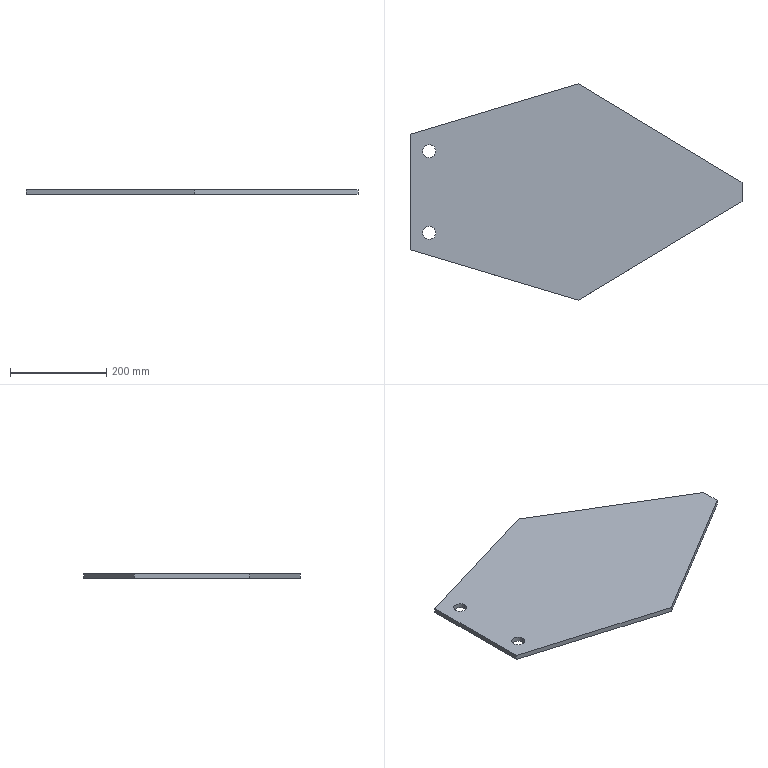Part | SolidWorks | features Extrusion 1, ICE 1 | 1 solid | 12 faces | box 690 x 450 x 10 mm | volume 2029049 mm3 | plane 8 | cylinder 4 | commonest cylinder face diameters 27 x4
STEP:
#1=CARTESIAN_POINT('',(-318.5,85.,0.));
#2=VERTEX_POINT('',#1);
#3=CARTESIAN_POINT('',(-291.5,85.,0.));
#4=VERTEX_POINT('',#3);
#5=CARTESIAN_POINT('',(-305.,85.,0.));
#6=DIRECTION('',(0.,0.,1.));
#7=DIRECTION('',(1.,0.,0.));
#8=AXIS2_PLACEMENT_3D('',#5,#6,#7);
#9=CIRCLE('',#8,13.5);
#10=EDGE_CURVE('',#2,#4,#9,.T.);
#11=ORIENTED_EDGE('',*,*,#10,.F.);
#12=CARTESIAN_POINT('',(-318.5,85.,10.));
#13=VERTEX_POINT('',#12);
#14=CARTESIAN_POINT('',(-318.5,85.,0.));
#15=DIRECTION('',(0.,0.,1.));
#16=VECTOR('',#15,1000.);
#17=LINE('',#14,#16);
#18=EDGE_CURVE('',#2,#13,#17,.T.);
#19=ORIENTED_EDGE('',*,*,#18,.T.);
#20=CARTESIAN_POINT('',(-291.5,85.,10.));
#21=VERTEX_POINT('',#20);
#22=CARTESIAN_POINT('',(-305.,85.,10.));
#23=DIRECTION('',(0.,0.,1.));
#24=DIRECTION('',(1.,0.,0.));
#25=AXIS2_PLACEMENT_3D('',#22,#23,#24);
#26=CIRCLE('',#25,13.5);
#27=EDGE_CURVE('',#13,#21,#26,.T.);
#28=ORIENTED_EDGE('',*,*,#27,.T.);
#29=CARTESIAN_POINT('',(-291.5,85.,0.));
#30=DIRECTION('',(0.,0.,1.));
#31=VECTOR('',#30,1000.);
#32=LINE('',#29,#31);
#33=EDGE_CURVE('',#4,#21,#32,.T.);
#34=ORIENTED_EDGE('',*,*,#33,.F.);
#35=EDGE_LOOP('',(#11,#19,#28,#34));
#36=FACE_OUTER_BOUND('',#35,.T.);
#37=CARTESIAN_POINT('',(-305.,85.,0.));
#38=DIRECTION('',(0.,0.,1.));
#39=DIRECTION('',(1.,0.,0.));
#40=AXIS2_PLACEMENT_3D('',#37,#38,#39);
#41=CYLINDRICAL_SURFACE('',#40,13.5);
#42=ADVANCED_FACE('',(#36),#41,.F.);
#43=CARTESIAN_POINT('',(-318.5,-85.,0.));
#44=VERTEX_POINT('',#43);
#45=CARTESIAN_POINT('',(-291.5,-85.,0.));
#46=VERTEX_POINT('',#45);
#47=CARTESIAN_POINT('',(-305.,-85.,0.));
#48=DIRECTION('',(0.,0.,1.));
#49=DIRECTION('',(1.,0.,0.));
#50=AXIS2_PLACEMENT_3D('',#47,#48,#49);
#51=CIRCLE('',#50,13.5);
#52=EDGE_CURVE('',#44,#46,#51,.T.);
#53=ORIENTED_EDGE('',*,*,#52,.F.);
#54=CARTESIAN_POINT('',(-318.5,-85.,10.));
#55=VERTEX_POINT('',#54);
#56=CARTESIAN_POINT('',(-318.5,-85.,0.));
#57=DIRECTION('',(0.,0.,1.));
#58=VECTOR('',#57,1000.);
#59=LINE('',#56,#58);
#60=EDGE_CURVE('',#44,#55,#59,.T.);
#61=ORIENTED_EDGE('',*,*,#60,.T.);
#62=CARTESIAN_POINT('',(-291.5,-85.,10.));
#63=VERTEX_POINT('',#62);
#64=CARTESIAN_POINT('',(-305.,-85.,10.));
#65=DIRECTION('',(0.,0.,1.));
#66=DIRECTION('',(1.,0.,0.));
#67=AXIS2_PLACEMENT_3D('',#64,#65,#66);
#68=CIRCLE('',#67,13.5);
#69=EDGE_CURVE('',#55,#63,#68,.T.);
#70=ORIENTED_EDGE('',*,*,#69,.T.);
#71=CARTESIAN_POINT('',(-291.5,-85.,0.));
#72=DIRECTION('',(0.,0.,1.));
#73=VECTOR('',#72,1000.);
#74=LINE('',#71,#73);
#75=EDGE_CURVE('',#46,#63,#74,.T.);
#76=ORIENTED_EDGE('',*,*,#75,.F.);
#77=EDGE_LOOP('',(#53,#61,#70,#76));
#78=FACE_OUTER_BOUND('',#77,.T.);
#79=CARTESIAN_POINT('',(-305.,-85.,0.));
#80=DIRECTION('',(0.,0.,1.));
#81=DIRECTION('',(1.,0.,0.));
#82=AXIS2_PLACEMENT_3D('',#79,#80,#81);
#83=CYLINDRICAL_SURFACE('',#82,13.5);
#84=ADVANCED_FACE('',(#78),#83,.F.);
#85=CARTESIAN_POINT('',(-345.,120.,10.));
#86=VERTEX_POINT('',#85);
#87=CARTESIAN_POINT('',(5.,225.,10.));
#88=VERTEX_POINT('',#87);
#89=CARTESIAN_POINT('',(-61.514,205.046,10.));
#90=DIRECTION('',(0.9578,0.2873,0.));
#91=VECTOR('',#90,1000.);
#92=LINE('',#89,#91);
#93=EDGE_CURVE('',#86,#88,#92,.T.);
#94=ORIENTED_EDGE('',*,*,#93,.F.);
#95=CARTESIAN_POINT('',(-345.,-120.,10.));
#96=VERTEX_POINT('',#95);
#97=CARTESIAN_POINT('',(-345.,-225.,10.));
#98=DIRECTION('',(0.,-1.,0.));
#99=VECTOR('',#98,1000.);
#100=LINE('',#97,#99);
#101=EDGE_CURVE('',#86,#96,#100,.T.);
#102=ORIENTED_EDGE('',*,*,#101,.T.);
#103=CARTESIAN_POINT('',(5.,-225.,10.));
#104=VERTEX_POINT('',#103);
#105=CARTESIAN_POINT('',(-61.514,-205.046,10.));
#106=DIRECTION('',(0.9578,-0.2873,0.));
#107=VECTOR('',#106,1000.);
#108=LINE('',#105,#107);
#109=EDGE_CURVE('',#96,#104,#108,.T.);
#110=ORIENTED_EDGE('',*,*,#109,.T.);
#111=CARTESIAN_POINT('',(345.,-20.,10.));
#112=VERTEX_POINT('',#111);
#113=CARTESIAN_POINT('',(100.826,-167.223,10.));
#114=DIRECTION('',(0.8564,0.5163,0.));
#115=VECTOR('',#114,1000.);
#116=LINE('',#113,#115);
#117=EDGE_CURVE('',#104,#112,#116,.T.);
#118=ORIENTED_EDGE('',*,*,#117,.T.);
#119=CARTESIAN_POINT('',(345.,20.,10.));
#120=VERTEX_POINT('',#119);
#121=CARTESIAN_POINT('',(345.,-225.,10.));
#122=DIRECTION('',(0.,1.,0.));
#123=VECTOR('',#122,1000.);
#124=LINE('',#121,#123);
#125=EDGE_CURVE('',#112,#120,#124,.T.);
#126=ORIENTED_EDGE('',*,*,#125,.T.);
#127=CARTESIAN_POINT('',(100.826,167.223,10.));
#128=DIRECTION('',(0.8564,-0.5163,0.));
#129=VECTOR('',#128,1000.);
#130=LINE('',#127,#129);
#131=EDGE_CURVE('',#88,#120,#130,.T.);
#132=ORIENTED_EDGE('',*,*,#131,.F.);
#133=EDGE_LOOP('',(#94,#102,#110,#118,#126,#132));
#134=FACE_OUTER_BOUND('',#133,.T.);
#135=CARTESIAN_POINT('',(-305.,85.,10.));
#136=DIRECTION('',(0.,0.,1.));
#137=DIRECTION('',(1.,0.,0.));
#138=AXIS2_PLACEMENT_3D('',#135,#136,#137);
#139=CIRCLE('',#138,13.5);
#140=EDGE_CURVE('',#21,#13,#139,.T.);
#141=ORIENTED_EDGE('',*,*,#140,.F.);
#142=ORIENTED_EDGE('',*,*,#27,.F.);
#143=EDGE_LOOP('',(#141,#142));
#144=FACE_BOUND('',#143,.T.);
#145=CARTESIAN_POINT('',(-305.,-85.,10.));
#146=DIRECTION('',(0.,0.,1.));
#147=DIRECTION('',(1.,0.,0.));
#148=AXIS2_PLACEMENT_3D('',#145,#146,#147);
#149=CIRCLE('',#148,13.5);
#150=EDGE_CURVE('',#63,#55,#149,.T.);
#151=ORIENTED_EDGE('',*,*,#150,.F.);
#152=ORIENTED_EDGE('',*,*,#69,.F.);
#153=EDGE_LOOP('',(#151,#152));
#154=FACE_BOUND('',#153,.T.);
#155=CARTESIAN_POINT('',(0.,0.,10.));
#156=DIRECTION('',(0.,0.,1.));
#157=DIRECTION('',(1.,0.,0.));
#158=AXIS2_PLACEMENT_3D('',#155,#156,#157);
#159=PLANE('',#158);
#160=ADVANCED_FACE('',(#134,#144,#154),#159,.T.);
#161=CARTESIAN_POINT('',(-305.,-85.,0.));
#162=DIRECTION('',(0.,0.,1.));
#163=DIRECTION('',(1.,0.,0.));
#164=AXIS2_PLACEMENT_3D('',#161,#162,#163);
#165=CIRCLE('',#164,13.5);
#166=EDGE_CURVE('',#46,#44,#165,.T.);
#167=ORIENTED_EDGE('',*,*,#166,.T.);
#168=ORIENTED_EDGE('',*,*,#52,.T.);
#169=EDGE_LOOP('',(#167,#168));
#170=FACE_BOUND('',#169,.T.);
#171=CARTESIAN_POINT('',(-305.,85.,0.));
#172=DIRECTION('',(0.,0.,1.));
#173=DIRECTION('',(1.,0.,0.));
#174=AXIS2_PLACEMENT_3D('',#171,#172,#173);
#175=CIRCLE('',#174,13.5);
#176=EDGE_CURVE('',#4,#2,#175,.T.);
#177=ORIENTED_EDGE('',*,*,#176,.T.);
#178=ORIENTED_EDGE('',*,*,#10,.T.);
#179=EDGE_LOOP('',(#177,#178));
#180=FACE_BOUND('',#179,.T.);
#181=CARTESIAN_POINT('',(-345.,120.,0.));
#182=VERTEX_POINT('',#181);
#183=CARTESIAN_POINT('',(-345.,-120.,0.));
#184=VERTEX_POINT('',#183);
#185=CARTESIAN_POINT('',(-345.,-225.,0.));
#186=DIRECTION('',(0.,-1.,0.));
#187=VECTOR('',#186,1000.);
#188=LINE('',#185,#187);
#189=EDGE_CURVE('',#182,#184,#188,.T.);
#190=ORIENTED_EDGE('',*,*,#189,.F.);
#191=CARTESIAN_POINT('',(5.,225.,0.));
#192=VERTEX_POINT('',#191);
#193=CARTESIAN_POINT('',(-61.514,205.046,0.));
#194=DIRECTION('',(0.9578,0.2873,0.));
#195=VECTOR('',#194,1000.);
#196=LINE('',#193,#195);
#197=EDGE_CURVE('',#182,#192,#196,.T.);
#198=ORIENTED_EDGE('',*,*,#197,.T.);
#199=CARTESIAN_POINT('',(345.,20.,0.));
#200=VERTEX_POINT('',#199);
#201=CARTESIAN_POINT('',(100.826,167.223,0.));
#202=DIRECTION('',(0.8564,-0.5163,0.));
#203=VECTOR('',#202,1000.);
#204=LINE('',#201,#203);
#205=EDGE_CURVE('',#192,#200,#204,.T.);
#206=ORIENTED_EDGE('',*,*,#205,.T.);
#207=CARTESIAN_POINT('',(345.,-20.,0.));
#208=VERTEX_POINT('',#207);
#209=CARTESIAN_POINT('',(345.,-225.,0.));
#210=DIRECTION('',(0.,1.,0.));
#211=VECTOR('',#210,1000.);
#212=LINE('',#209,#211);
#213=EDGE_CURVE('',#208,#200,#212,.T.);
#214=ORIENTED_EDGE('',*,*,#213,.F.);
#215=CARTESIAN_POINT('',(5.,-225.,0.));
#216=VERTEX_POINT('',#215);
#217=CARTESIAN_POINT('',(100.826,-167.223,0.));
#218=DIRECTION('',(0.8564,0.5163,0.));
#219=VECTOR('',#218,1000.);
#220=LINE('',#217,#219);
#221=EDGE_CURVE('',#216,#208,#220,.T.);
#222=ORIENTED_EDGE('',*,*,#221,.F.);
#223=CARTESIAN_POINT('',(-61.514,-205.046,0.));
#224=DIRECTION('',(0.9578,-0.2873,0.));
#225=VECTOR('',#224,1000.);
#226=LINE('',#223,#225);
#227=EDGE_CURVE('',#184,#216,#226,.T.);
#228=ORIENTED_EDGE('',*,*,#227,.F.);
#229=EDGE_LOOP('',(#190,#198,#206,#214,#222,#228));
#230=FACE_OUTER_BOUND('',#229,.T.);
#231=CARTESIAN_POINT('',(0.,0.,0.));
#232=DIRECTION('',(0.,0.,1.));
#233=DIRECTION('',(1.,0.,0.));
#234=AXIS2_PLACEMENT_3D('',#231,#232,#233);
#235=PLANE('',#234);
#236=ADVANCED_FACE('',(#170,#180,#230),#235,.F.);
#237=ORIENTED_EDGE('',*,*,#101,.F.);
#238=CARTESIAN_POINT('',(-345.,120.,0.));
#239=DIRECTION('',(0.,0.,1.));
#240=VECTOR('',#239,1000.);
#241=LINE('',#238,#240);
#242=EDGE_CURVE('',#182,#86,#241,.T.);
#243=ORIENTED_EDGE('',*,*,#242,.F.);
#244=ORIENTED_EDGE('',*,*,#189,.T.);
#245=CARTESIAN_POINT('',(-345.,-120.,0.));
#246=DIRECTION('',(0.,0.,1.));
#247=VECTOR('',#246,1000.);
#248=LINE('',#245,#247);
#249=EDGE_CURVE('',#184,#96,#248,.T.);
#250=ORIENTED_EDGE('',*,*,#249,.T.);
#251=EDGE_LOOP('',(#237,#243,#244,#250));
#252=FACE_OUTER_BOUND('',#251,.T.);
#253=CARTESIAN_POINT('',(-345.,-225.,10.));
#254=DIRECTION('',(1.,0.,0.));
#255=DIRECTION('',(0.,0.,-1.));
#256=AXIS2_PLACEMENT_3D('',#253,#254,#255);
#257=PLANE('',#256);
#258=ADVANCED_FACE('',(#252),#257,.F.);
#259=CARTESIAN_POINT('',(345.,-20.,0.));
#260=DIRECTION('',(0.,0.,1.));
#261=VECTOR('',#260,1000.);
#262=LINE('',#259,#261);
#263=EDGE_CURVE('',#208,#112,#262,.T.);
#264=ORIENTED_EDGE('',*,*,#263,.F.);
#265=ORIENTED_EDGE('',*,*,#213,.T.);
#266=CARTESIAN_POINT('',(345.,20.,0.));
#267=DIRECTION('',(0.,0.,1.));
#268=VECTOR('',#267,1000.);
#269=LINE('',#266,#268);
#270=EDGE_CURVE('',#200,#120,#269,.T.);
#271=ORIENTED_EDGE('',*,*,#270,.T.);
#272=ORIENTED_EDGE('',*,*,#125,.F.);
#273=EDGE_LOOP('',(#264,#265,#271,#272));
#274=FACE_OUTER_BOUND('',#273,.T.);
#275=CARTESIAN_POINT('',(345.,-225.,10.));
#276=DIRECTION('',(-1.,0.,0.));
#277=DIRECTION('',(0.,0.,1.));
#278=AXIS2_PLACEMENT_3D('',#275,#276,#277);
#279=PLANE('',#278);
#280=ADVANCED_FACE('',(#274),#279,.F.);
#281=ORIENTED_EDGE('',*,*,#131,.T.);
#282=ORIENTED_EDGE('',*,*,#270,.F.);
#283=ORIENTED_EDGE('',*,*,#205,.F.);
#284=CARTESIAN_POINT('',(5.,225.,0.));
#285=DIRECTION('',(0.,0.,1.));
#286=VECTOR('',#285,1000.);
#287=LINE('',#284,#286);
#288=EDGE_CURVE('',#192,#88,#287,.T.);
#289=ORIENTED_EDGE('',*,*,#288,.T.);
#290=EDGE_LOOP('',(#281,#282,#283,#289));
#291=FACE_OUTER_BOUND('',#290,.T.);
#292=CARTESIAN_POINT('',(100.826,167.223,0.));
#293=DIRECTION('',(-0.5163,-0.8564,0.));
#294=DIRECTION('',(0.8564,-0.5163,0.));
#295=AXIS2_PLACEMENT_3D('',#292,#293,#294);
#296=PLANE('',#295);
#297=ADVANCED_FACE('',(#291),#296,.F.);
#298=ORIENTED_EDGE('',*,*,#117,.F.);
#299=CARTESIAN_POINT('',(5.,-225.,0.));
#300=DIRECTION('',(0.,0.,1.));
#301=VECTOR('',#300,1000.);
#302=LINE('',#299,#301);
#303=EDGE_CURVE('',#216,#104,#302,.T.);
#304=ORIENTED_EDGE('',*,*,#303,.F.);
#305=ORIENTED_EDGE('',*,*,#221,.T.);
#306=ORIENTED_EDGE('',*,*,#263,.T.);
#307=EDGE_LOOP('',(#298,#304,#305,#306));
#308=FACE_OUTER_BOUND('',#307,.T.);
#309=CARTESIAN_POINT('',(100.826,-167.223,0.));
#310=DIRECTION('',(0.5163,-0.8564,0.));
#311=DIRECTION('',(0.8564,0.5163,0.));
#312=AXIS2_PLACEMENT_3D('',#309,#310,#311);
#313=PLANE('',#312);
#314=ADVANCED_FACE('',(#308),#313,.T.);
#315=ORIENTED_EDGE('',*,*,#60,.F.);
#316=ORIENTED_EDGE('',*,*,#166,.F.);
#317=ORIENTED_EDGE('',*,*,#75,.T.);
#318=ORIENTED_EDGE('',*,*,#150,.T.);
#319=EDGE_LOOP('',(#315,#316,#317,#318));
#320=FACE_OUTER_BOUND('',#319,.T.);
#321=CARTESIAN_POINT('',(-305.,-85.,0.));
#322=DIRECTION('',(0.,0.,1.));
#323=DIRECTION('',(1.,0.,0.));
#324=AXIS2_PLACEMENT_3D('',#321,#322,#323);
#325=CYLINDRICAL_SURFACE('',#324,13.5);
#326=ADVANCED_FACE('',(#320),#325,.F.);
#327=ORIENTED_EDGE('',*,*,#18,.F.);
#328=ORIENTED_EDGE('',*,*,#176,.F.);
#329=ORIENTED_EDGE('',*,*,#33,.T.);
#330=ORIENTED_EDGE('',*,*,#140,.T.);
#331=EDGE_LOOP('',(#327,#328,#329,#330));
#332=FACE_OUTER_BOUND('',#331,.T.);
#333=CARTESIAN_POINT('',(-305.,85.,0.));
#334=DIRECTION('',(0.,0.,1.));
#335=DIRECTION('',(1.,0.,0.));
#336=AXIS2_PLACEMENT_3D('',#333,#334,#335);
#337=CYLINDRICAL_SURFACE('',#336,13.5);
#338=ADVANCED_FACE('',(#332),#337,.F.);
#339=ORIENTED_EDGE('',*,*,#109,.F.);
#340=ORIENTED_EDGE('',*,*,#249,.F.);
#341=ORIENTED_EDGE('',*,*,#227,.T.);
#342=ORIENTED_EDGE('',*,*,#303,.T.);
#343=EDGE_LOOP('',(#339,#340,#341,#342));
#344=FACE_OUTER_BOUND('',#343,.T.);
#345=CARTESIAN_POINT('',(-61.514,-205.046,0.));
#346=DIRECTION('',(-0.2873,-0.9578,0.));
#347=DIRECTION('',(0.9578,-0.2873,0.));
#348=AXIS2_PLACEMENT_3D('',#345,#346,#347);
#349=PLANE('',#348);
#350=ADVANCED_FACE('',(#344),#349,.T.);
#351=ORIENTED_EDGE('',*,*,#93,.T.);
#352=ORIENTED_EDGE('',*,*,#288,.F.);
#353=ORIENTED_EDGE('',*,*,#197,.F.);
#354=ORIENTED_EDGE('',*,*,#242,.T.);
#355=EDGE_LOOP('',(#351,#352,#353,#354));
#356=FACE_OUTER_BOUND('',#355,.T.);
#357=CARTESIAN_POINT('',(-61.514,205.046,0.));
#358=DIRECTION('',(0.2873,-0.9578,0.));
#359=DIRECTION('',(0.9578,0.2873,0.));
#360=AXIS2_PLACEMENT_3D('',#357,#358,#359);
#361=PLANE('',#360);
#362=ADVANCED_FACE('',(#356),#361,.F.);
#363=CLOSED_SHELL('',(#42,#84,#160,#236,#258,#280,#297,#314,#326,#338,#350,#362));
#364=MANIFOLD_SOLID_BREP('',#363);
#365=CARTESIAN_POINT('',(0.,0.,0.));
#366=DIRECTION('',(0.,0.,1.));
#367=DIRECTION('',(1.,0.,0.));
#368=AXIS2_PLACEMENT_3D('',#365,#366,#367);
#369=(LENGTH_UNIT()NAMED_UNIT(*)SI_UNIT(.MILLI.,.METRE.));
#370=UNCERTAINTY_MEASURE_WITH_UNIT(LENGTH_MEASURE(0.00001),#369,'','');
#371=(NAMED_UNIT(*)PLANE_ANGLE_UNIT()SI_UNIT($,.RADIAN.));
#372=(NAMED_UNIT(*)SI_UNIT($,.STERADIAN.)SOLID_ANGLE_UNIT());
#373=(GEOMETRIC_REPRESENTATION_CONTEXT(3)GLOBAL_UNCERTAINTY_ASSIGNED_CONTEXT((#370))GLOBAL_UNIT_ASSIGNED_CONTEXT((#369,#371,#372))REPRESENTATION_CONTEXT('',''));
#374=ADVANCED_BREP_SHAPE_REPRESENTATION('',(#364,#368),#373);